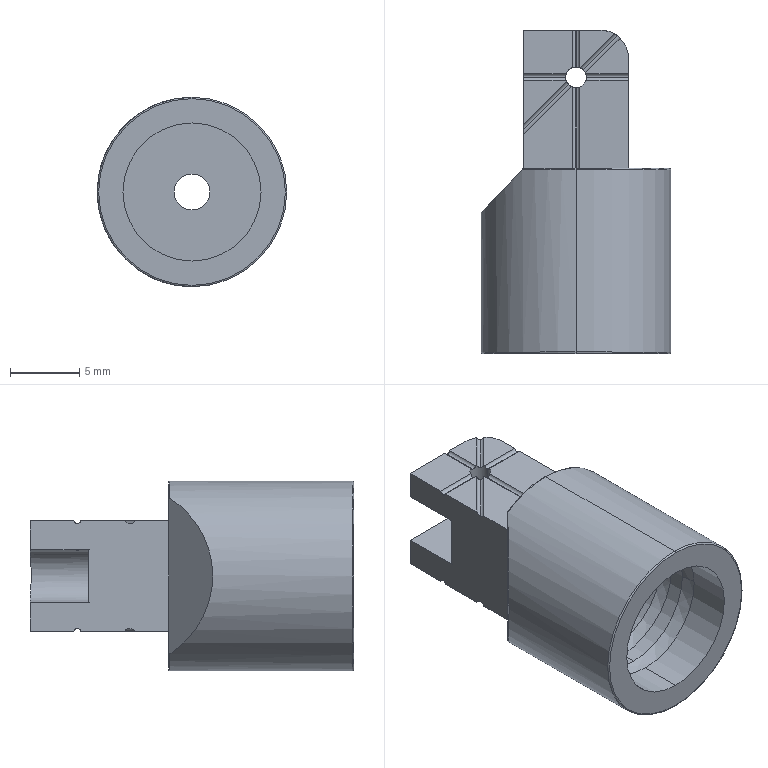Part | SolidWorks | features ICE 7, Fillet 2, MirrorPattern 1, Revolution 1 | 1 solid | 87 faces | box 13.72 x 23.4 x 13.72 mm | volume 1526 mm3 | cylinder 40 | plane 38 | torus 5 | spline 4 | commonest cylinder face diameters 0.51 x24 10 x6 1.5 x4 2.6 x2 13.72 x2 3.85 x1